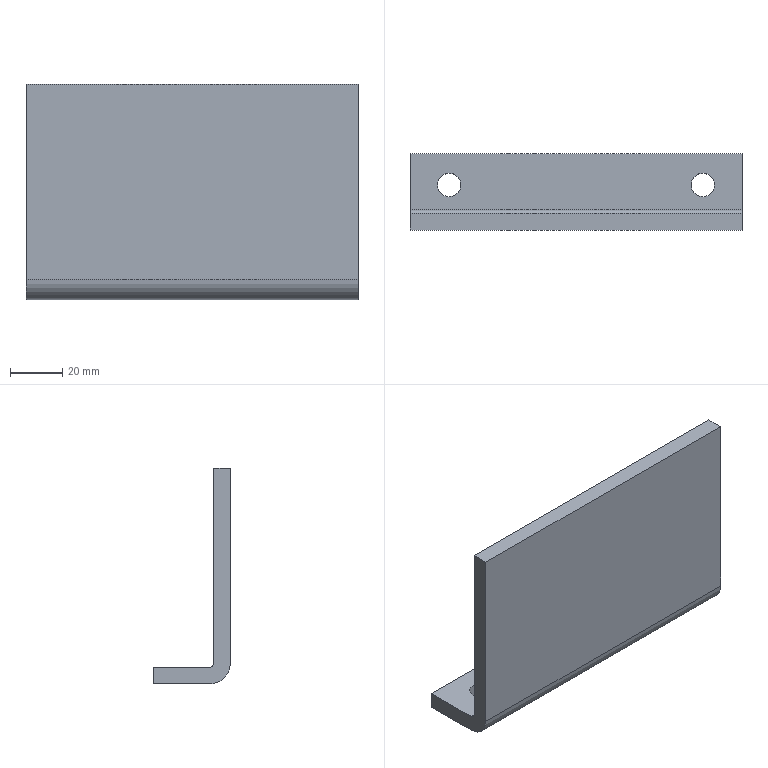Part | STEP file | 1_id706_x_t | 1 solid | 14 faces | box 127 x 29.369 x 82.55 mm | volume 82680 mm3 | plane 8 | cylinder 6 | commonest cylinder face diameters 9 x4 3.175 x1 15.875 x1
STEP:
#1=CARTESIAN_POINT('',(0.,0.,0.));
#2=DIRECTION('',(0.,0.,1.));
#3=DIRECTION('',(1.,0.,0.));
#4=AXIS2_PLACEMENT_3D('',#1,#2,#3);
#5=CARTESIAN_POINT('',(412.638,-208.869,-45.55));
#6=VERTEX_POINT('',#5);
#7=CARTESIAN_POINT('',(412.638,-202.519,-45.55));
#8=VERTEX_POINT('',#7);
#9=CARTESIAN_POINT('',(412.638,-208.869,-45.55));
#10=DIRECTION('',(0.,1.,0.));
#11=VECTOR('',#10,1.);
#12=LINE('',#9,#11);
#13=CARTESIAN_POINT('',(476.138,-148.544,-45.55));
#14=DIRECTION('',(0.,0.,1.));
#15=DIRECTION('',(1.,0.,0.));
#16=AXIS2_PLACEMENT_3D('',#13,#14,#15);
#17=PLANE('',#16);
#18=CARTESIAN_POINT('',(-63.5,-60.325));
#19=DIRECTION('',(0.,1.));
#20=VECTOR('',#19,1.);
#21=LINE('',#18,#20);
#22=(GEOMETRIC_REPRESENTATION_CONTEXT(2)PARAMETRIC_REPRESENTATION_CONTEXT()REPRESENTATION_CONTEXT('',''));
#23=DEFINITIONAL_REPRESENTATION('',(#21),#22);
#24=PCURVE('',#17,#23);
#25=CARTESIAN_POINT('',(412.638,-148.544,-86.825));
#26=DIRECTION('',(-1.,0.,0.));
#27=DIRECTION('',(0.,-1.,0.));
#28=AXIS2_PLACEMENT_3D('',#25,#26,#27);
#29=PLANE('',#28);
#30=CARTESIAN_POINT('',(60.325,41.275));
#31=DIRECTION('',(-1.,0.));
#32=VECTOR('',#31,1.);
#33=LINE('',#30,#32);
#34=(GEOMETRIC_REPRESENTATION_CONTEXT(2)PARAMETRIC_REPRESENTATION_CONTEXT()REPRESENTATION_CONTEXT('',''));
#35=DEFINITIONAL_REPRESENTATION('',(#33),#34);
#36=PCURVE('',#29,#35);
#37=SURFACE_CURVE('',#12,(#24,#36),.PCURVE_S1.);
#38=EDGE_CURVE('',#6,#8,#37,.T.);
#39=ORIENTED_EDGE('',*,*,#38,.F.);
#40=CARTESIAN_POINT('',(539.638,-208.869,-45.55));
#41=VERTEX_POINT('',#40);
#42=CARTESIAN_POINT('',(412.638,-208.869,-45.55));
#43=DIRECTION('',(1.,0.,0.));
#44=VECTOR('',#43,1.);
#45=LINE('',#42,#44);
#46=CARTESIAN_POINT('',(-63.5,-60.325));
#47=DIRECTION('',(1.,0.));
#48=VECTOR('',#47,1.);
#49=LINE('',#46,#48);
#50=(GEOMETRIC_REPRESENTATION_CONTEXT(2)PARAMETRIC_REPRESENTATION_CONTEXT()REPRESENTATION_CONTEXT('',''));
#51=DEFINITIONAL_REPRESENTATION('',(#49),#50);
#52=PCURVE('',#17,#51);
#53=CARTESIAN_POINT('',(476.138,-208.869,-86.825));
#54=DIRECTION('',(0.,-1.,0.));
#55=DIRECTION('',(0.,0.,1.));
#56=AXIS2_PLACEMENT_3D('',#53,#54,#55);
#57=PLANE('',#56);
#58=CARTESIAN_POINT('',(41.275,63.5));
#59=DIRECTION('',(0.,-1.));
#60=VECTOR('',#59,1.);
#61=LINE('',#58,#60);
#62=(GEOMETRIC_REPRESENTATION_CONTEXT(2)PARAMETRIC_REPRESENTATION_CONTEXT()REPRESENTATION_CONTEXT('',''));
#63=DEFINITIONAL_REPRESENTATION('',(#61),#62);
#64=PCURVE('',#57,#63);
#65=SURFACE_CURVE('',#45,(#52,#64),.PCURVE_S1.);
#66=EDGE_CURVE('',#6,#41,#65,.T.);
#67=ORIENTED_EDGE('',*,*,#66,.T.);
#68=CARTESIAN_POINT('',(539.638,-202.519,-45.55));
#69=VERTEX_POINT('',#68);
#70=CARTESIAN_POINT('',(539.638,-208.869,-45.55));
#71=DIRECTION('',(0.,1.,0.));
#72=VECTOR('',#71,1.);
#73=LINE('',#70,#72);
#74=CARTESIAN_POINT('',(63.5,-60.325));
#75=DIRECTION('',(0.,1.));
#76=VECTOR('',#75,1.);
#77=LINE('',#74,#76);
#78=(GEOMETRIC_REPRESENTATION_CONTEXT(2)PARAMETRIC_REPRESENTATION_CONTEXT()REPRESENTATION_CONTEXT('',''));
#79=DEFINITIONAL_REPRESENTATION('',(#77),#78);
#80=PCURVE('',#17,#79);
#81=CARTESIAN_POINT('',(539.638,-148.544,-86.825));
#82=DIRECTION('',(1.,0.,0.));
#83=DIRECTION('',(0.,0.,-1.));
#84=AXIS2_PLACEMENT_3D('',#81,#82,#83);
#85=PLANE('',#84);
#86=CARTESIAN_POINT('',(-41.275,-60.325));
#87=DIRECTION('',(0.,1.));
#88=VECTOR('',#87,1.);
#89=LINE('',#86,#88);
#90=(GEOMETRIC_REPRESENTATION_CONTEXT(2)PARAMETRIC_REPRESENTATION_CONTEXT()REPRESENTATION_CONTEXT('',''));
#91=DEFINITIONAL_REPRESENTATION('',(#89),#90);
#92=PCURVE('',#85,#91);
#93=SURFACE_CURVE('',#73,(#80,#92),.PCURVE_S1.);
#94=EDGE_CURVE('',#41,#69,#93,.T.);
#95=ORIENTED_EDGE('',*,*,#94,.T.);
#96=CARTESIAN_POINT('',(412.638,-202.519,-45.55));
#97=DIRECTION('',(1.,0.,0.));
#98=VECTOR('',#97,1.);
#99=LINE('',#96,#98);
#100=CARTESIAN_POINT('',(-63.5,-53.975));
#101=DIRECTION('',(1.,0.));
#102=VECTOR('',#101,1.);
#103=LINE('',#100,#102);
#104=(GEOMETRIC_REPRESENTATION_CONTEXT(2)PARAMETRIC_REPRESENTATION_CONTEXT()REPRESENTATION_CONTEXT('',''));
#105=DEFINITIONAL_REPRESENTATION('',(#103),#104);
#106=PCURVE('',#17,#105);
#107=CARTESIAN_POINT('',(476.138,-202.519,-86.825));
#108=DIRECTION('',(0.,-1.,0.));
#109=DIRECTION('',(0.,0.,1.));
#110=AXIS2_PLACEMENT_3D('',#107,#108,#109);
#111=PLANE('',#110);
#112=CARTESIAN_POINT('',(41.275,63.5));
#113=DIRECTION('',(0.,-1.));
#114=VECTOR('',#113,1.);
#115=LINE('',#112,#114);
#116=(GEOMETRIC_REPRESENTATION_CONTEXT(2)PARAMETRIC_REPRESENTATION_CONTEXT()REPRESENTATION_CONTEXT('',''));
#117=DEFINITIONAL_REPRESENTATION('',(#115),#116);
#118=PCURVE('',#111,#117);
#119=SURFACE_CURVE('',#99,(#106,#118),.PCURVE_S1.);
#120=EDGE_CURVE('',#8,#69,#119,.T.);
#121=ORIENTED_EDGE('',*,*,#120,.F.);
#122=EDGE_LOOP('',(#39,#67,#95,#121));
#123=FACE_BOUND('',#122,.T.);
#124=ADVANCED_FACE('',(#123),#17,.T.);
#125=ORIENTED_EDGE('',*,*,#120,.T.);
#126=CARTESIAN_POINT('',(539.638,-202.519,-120.163));
#127=VERTEX_POINT('',#126);
#128=CARTESIAN_POINT('',(539.638,-202.519,-45.55));
#129=DIRECTION('',(0.,0.,-1.));
#130=VECTOR('',#129,1.);
#131=LINE('',#128,#130);
#132=CARTESIAN_POINT('',(41.275,-63.5));
#133=DIRECTION('',(-1.,0.));
#134=VECTOR('',#133,1.);
#135=LINE('',#132,#134);
#136=(GEOMETRIC_REPRESENTATION_CONTEXT(2)PARAMETRIC_REPRESENTATION_CONTEXT()REPRESENTATION_CONTEXT('',''));
#137=DEFINITIONAL_REPRESENTATION('',(#135),#136);
#138=PCURVE('',#111,#137);
#139=CARTESIAN_POINT('',(-41.275,-53.975));
#140=DIRECTION('',(1.,0.));
#141=VECTOR('',#140,1.);
#142=LINE('',#139,#141);
#143=(GEOMETRIC_REPRESENTATION_CONTEXT(2)PARAMETRIC_REPRESENTATION_CONTEXT()REPRESENTATION_CONTEXT('',''));
#144=DEFINITIONAL_REPRESENTATION('',(#142),#143);
#145=PCURVE('',#85,#144);
#146=SURFACE_CURVE('',#131,(#138,#145),.PCURVE_S1.);
#147=EDGE_CURVE('',#69,#127,#146,.T.);
#148=ORIENTED_EDGE('',*,*,#147,.T.);
#149=CARTESIAN_POINT('',(412.638,-202.519,-120.163));
#150=VERTEX_POINT('',#149);
#151=CARTESIAN_POINT('',(412.638,-202.519,-120.163));
#152=DIRECTION('',(1.,0.,0.));
#153=VECTOR('',#152,1.);
#154=LINE('',#151,#153);
#155=CARTESIAN_POINT('',(-33.337,63.5));
#156=DIRECTION('',(0.,-1.));
#157=VECTOR('',#156,1.);
#158=LINE('',#155,#157);
#159=(GEOMETRIC_REPRESENTATION_CONTEXT(2)PARAMETRIC_REPRESENTATION_CONTEXT()REPRESENTATION_CONTEXT('',''));
#160=DEFINITIONAL_REPRESENTATION('',(#158),#159);
#161=PCURVE('',#111,#160);
#162=CARTESIAN_POINT('',(476.138,-200.931,-120.163));
#163=DIRECTION('',(1.,0.,0.));
#164=DIRECTION('',(0.,-1.,0.));
#165=AXIS2_PLACEMENT_3D('',#162,#163,#164);
#166=CYLINDRICAL_SURFACE('',#165,1.587);
#167=CARTESIAN_POINT('',(0.,-63.5));
#168=DIRECTION('',(0.,1.));
#169=VECTOR('',#168,1.);
#170=LINE('',#167,#169);
#171=(GEOMETRIC_REPRESENTATION_CONTEXT(2)PARAMETRIC_REPRESENTATION_CONTEXT()REPRESENTATION_CONTEXT('',''));
#172=DEFINITIONAL_REPRESENTATION('',(#170),#171);
#173=PCURVE('',#166,#172);
#174=SURFACE_CURVE('',#154,(#161,#173),.PCURVE_S1.);
#175=EDGE_CURVE('',#150,#127,#174,.T.);
#176=ORIENTED_EDGE('',*,*,#175,.F.);
#177=CARTESIAN_POINT('',(412.638,-202.519,-120.163));
#178=DIRECTION('',(0.,0.,1.));
#179=VECTOR('',#178,1.);
#180=LINE('',#177,#179);
#181=CARTESIAN_POINT('',(-33.337,63.5));
#182=DIRECTION('',(1.,0.));
#183=VECTOR('',#182,1.);
#184=LINE('',#181,#183);
#185=(GEOMETRIC_REPRESENTATION_CONTEXT(2)PARAMETRIC_REPRESENTATION_CONTEXT()REPRESENTATION_CONTEXT('',''));
#186=DEFINITIONAL_REPRESENTATION('',(#184),#185);
#187=PCURVE('',#111,#186);
#188=CARTESIAN_POINT('',(53.975,-33.337));
#189=DIRECTION('',(0.,1.));
#190=VECTOR('',#189,1.);
#191=LINE('',#188,#190);
#192=(GEOMETRIC_REPRESENTATION_CONTEXT(2)PARAMETRIC_REPRESENTATION_CONTEXT()REPRESENTATION_CONTEXT('',''));
#193=DEFINITIONAL_REPRESENTATION('',(#191),#192);
#194=PCURVE('',#29,#193);
#195=SURFACE_CURVE('',#180,(#187,#194),.PCURVE_S1.);
#196=EDGE_CURVE('',#150,#8,#195,.T.);
#197=ORIENTED_EDGE('',*,*,#196,.T.);
#198=EDGE_LOOP('',(#125,#148,#176,#197));
#199=FACE_BOUND('',#198,.T.);
#200=ADVANCED_FACE('',(#199),#111,.F.);
#201=CARTESIAN_POINT('',(412.638,-200.931,-128.1));
#202=VERTEX_POINT('',#201);
#203=CARTESIAN_POINT('',(412.638,-179.5,-128.1));
#204=VERTEX_POINT('',#203);
#205=CARTESIAN_POINT('',(412.638,-200.931,-128.1));
#206=DIRECTION('',(0.,1.,0.));
#207=VECTOR('',#206,1.);
#208=LINE('',#205,#207);
#209=CARTESIAN_POINT('',(52.388,-41.275));
#210=DIRECTION('',(-1.,0.));
#211=VECTOR('',#210,1.);
#212=LINE('',#209,#211);
#213=(GEOMETRIC_REPRESENTATION_CONTEXT(2)PARAMETRIC_REPRESENTATION_CONTEXT()REPRESENTATION_CONTEXT('',''));
#214=DEFINITIONAL_REPRESENTATION('',(#212),#213);
#215=PCURVE('',#29,#214);
#216=CARTESIAN_POINT('',(476.138,-148.544,-128.1));
#217=DIRECTION('',(0.,0.,-1.));
#218=DIRECTION('',(0.,1.,0.));
#219=AXIS2_PLACEMENT_3D('',#216,#217,#218);
#220=PLANE('',#219);
#221=CARTESIAN_POINT('',(-52.388,-63.5));
#222=DIRECTION('',(1.,0.));
#223=VECTOR('',#222,1.);
#224=LINE('',#221,#223);
#225=(GEOMETRIC_REPRESENTATION_CONTEXT(2)PARAMETRIC_REPRESENTATION_CONTEXT()REPRESENTATION_CONTEXT('',''));
#226=DEFINITIONAL_REPRESENTATION('',(#224),#225);
#227=PCURVE('',#220,#226);
#228=SURFACE_CURVE('',#208,(#215,#227),.PCURVE_S1.);
#229=EDGE_CURVE('',#202,#204,#228,.T.);
#230=ORIENTED_EDGE('',*,*,#229,.F.);
#231=CARTESIAN_POINT('',(412.638,-208.869,-120.163));
#232=VERTEX_POINT('',#231);
#233=CARTESIAN_POINT('',(412.638,-200.931,-120.163));
#234=DIRECTION('',(-1.,0.,0.));
#235=DIRECTION('',(0.,0.,-1.));
#236=AXIS2_PLACEMENT_3D('',#233,#234,#235);
#237=CIRCLE('',#236,7.938);
#238=CARTESIAN_POINT('',(52.388,-33.337));
#239=DIRECTION('',(0.,-1.));
#240=AXIS2_PLACEMENT_2D('',#238,#239);
#241=CIRCLE('',#240,7.938);
#242=(GEOMETRIC_REPRESENTATION_CONTEXT(2)PARAMETRIC_REPRESENTATION_CONTEXT()REPRESENTATION_CONTEXT('',''));
#243=DEFINITIONAL_REPRESENTATION('',(#241),#242);
#244=PCURVE('',#29,#243);
#245=CARTESIAN_POINT('',(476.138,-200.931,-120.163));
#246=DIRECTION('',(-1.,0.,0.));
#247=DIRECTION('',(0.,1.,0.));
#248=AXIS2_PLACEMENT_3D('',#245,#246,#247);
#249=CYLINDRICAL_SURFACE('',#248,7.938);
#250=CARTESIAN_POINT('',(1.571,63.5));
#251=DIRECTION('',(1.,0.));
#252=VECTOR('',#251,1.);
#253=LINE('',#250,#252);
#254=(GEOMETRIC_REPRESENTATION_CONTEXT(2)PARAMETRIC_REPRESENTATION_CONTEXT()REPRESENTATION_CONTEXT('',''));
#255=DEFINITIONAL_REPRESENTATION('',(#253),#254);
#256=PCURVE('',#249,#255);
#257=SURFACE_CURVE('',#237,(#244,#256),.PCURVE_S1.);
#258=EDGE_CURVE('',#202,#232,#257,.T.);
#259=ORIENTED_EDGE('',*,*,#258,.T.);
#260=CARTESIAN_POINT('',(412.638,-208.869,-120.163));
#261=DIRECTION('',(0.,0.,1.));
#262=VECTOR('',#261,1.);
#263=LINE('',#260,#262);
#264=CARTESIAN_POINT('',(60.325,-33.337));
#265=DIRECTION('',(0.,1.));
#266=VECTOR('',#265,1.);
#267=LINE('',#264,#266);
#268=(GEOMETRIC_REPRESENTATION_CONTEXT(2)PARAMETRIC_REPRESENTATION_CONTEXT()REPRESENTATION_CONTEXT('',''));
#269=DEFINITIONAL_REPRESENTATION('',(#267),#268);
#270=PCURVE('',#29,#269);
#271=CARTESIAN_POINT('',(-33.337,63.5));
#272=DIRECTION('',(1.,0.));
#273=VECTOR('',#272,1.);
#274=LINE('',#271,#273);
#275=(GEOMETRIC_REPRESENTATION_CONTEXT(2)PARAMETRIC_REPRESENTATION_CONTEXT()REPRESENTATION_CONTEXT('',''));
#276=DEFINITIONAL_REPRESENTATION('',(#274),#275);
#277=PCURVE('',#57,#276);
#278=SURFACE_CURVE('',#263,(#270,#277),.PCURVE_S1.);
#279=EDGE_CURVE('',#232,#6,#278,.T.);
#280=ORIENTED_EDGE('',*,*,#279,.T.);
#281=ORIENTED_EDGE('',*,*,#38,.T.);
#282=ORIENTED_EDGE('',*,*,#196,.F.);
#283=CARTESIAN_POINT('',(412.638,-200.931,-121.75));
#284=VERTEX_POINT('',#283);
#285=CARTESIAN_POINT('',(412.638,-200.931,-120.163));
#286=DIRECTION('',(1.,0.,0.));
#287=DIRECTION('',(0.,-1.,0.));
#288=AXIS2_PLACEMENT_3D('',#285,#286,#287);
#289=CIRCLE('',#288,1.587);
#290=CARTESIAN_POINT('',(53.975,-33.337));
#291=CARTESIAN_POINT('',(53.975,-36.087));
#292=CARTESIAN_POINT('',(51.594,-34.712));
#293=CARTESIAN_POINT('',(49.212,-33.337));
#294=CARTESIAN_POINT('',(51.594,-31.963));
#295=CARTESIAN_POINT('',(53.975,-30.588));
#296=CARTESIAN_POINT('',(53.975,-33.337));
#297=(BOUNDED_CURVE()B_SPLINE_CURVE(2,(#290,#291,#292,#293,#294,#295,#296),.UNSPECIFIED.,.T.,.F.)B_SPLINE_CURVE_WITH_KNOTS((1,2,2,2,2,1),(-2.094,0.,2.094,4.189,6.283,8.378),.UNSPECIFIED.)CURVE()GEOMETRIC_REPRESENTATION_ITEM()RATIONAL_B_SPLINE_CURVE((1.,0.5,1.,0.5,1.,0.5,1.))REPRESENTATION_ITEM(''));
#298=(GEOMETRIC_REPRESENTATION_CONTEXT(2)PARAMETRIC_REPRESENTATION_CONTEXT()REPRESENTATION_CONTEXT('',''));
#299=DEFINITIONAL_REPRESENTATION('',(#297),#298);
#300=PCURVE('',#29,#299);
#301=CARTESIAN_POINT('',(0.,-63.5));
#302=DIRECTION('',(1.,0.));
#303=VECTOR('',#302,1.);
#304=LINE('',#301,#303);
#305=(GEOMETRIC_REPRESENTATION_CONTEXT(2)PARAMETRIC_REPRESENTATION_CONTEXT()REPRESENTATION_CONTEXT('',''));
#306=DEFINITIONAL_REPRESENTATION('',(#304),#305);
#307=PCURVE('',#166,#306);
#308=SURFACE_CURVE('',#289,(#300,#307),.PCURVE_S1.);
#309=EDGE_CURVE('',#150,#284,#308,.T.);
#310=ORIENTED_EDGE('',*,*,#309,.T.);
#311=CARTESIAN_POINT('',(412.638,-179.5,-121.75));
#312=VERTEX_POINT('',#311);
#313=CARTESIAN_POINT('',(412.638,-200.931,-121.75));
#314=DIRECTION('',(0.,1.,0.));
#315=VECTOR('',#314,1.);
#316=LINE('',#313,#315);
#317=CARTESIAN_POINT('',(52.388,-34.925));
#318=DIRECTION('',(-1.,0.));
#319=VECTOR('',#318,1.);
#320=LINE('',#317,#319);
#321=(GEOMETRIC_REPRESENTATION_CONTEXT(2)PARAMETRIC_REPRESENTATION_CONTEXT()REPRESENTATION_CONTEXT('',''));
#322=DEFINITIONAL_REPRESENTATION('',(#320),#321);
#323=PCURVE('',#29,#322);
#324=CARTESIAN_POINT('',(476.138,-148.544,-121.75));
#325=DIRECTION('',(0.,0.,-1.));
#326=DIRECTION('',(0.,1.,0.));
#327=AXIS2_PLACEMENT_3D('',#324,#325,#326);
#328=PLANE('',#327);
#329=CARTESIAN_POINT('',(-52.388,-63.5));
#330=DIRECTION('',(1.,0.));
#331=VECTOR('',#330,1.);
#332=LINE('',#329,#331);
#333=(GEOMETRIC_REPRESENTATION_CONTEXT(2)PARAMETRIC_REPRESENTATION_CONTEXT()REPRESENTATION_CONTEXT('',''));
#334=DEFINITIONAL_REPRESENTATION('',(#332),#333);
#335=PCURVE('',#328,#334);
#336=SURFACE_CURVE('',#316,(#323,#335),.PCURVE_S1.);
#337=EDGE_CURVE('',#284,#312,#336,.T.);
#338=ORIENTED_EDGE('',*,*,#337,.T.);
#339=CARTESIAN_POINT('',(412.638,-179.5,-128.1));
#340=DIRECTION('',(0.,0.,1.));
#341=VECTOR('',#340,1.);
#342=LINE('',#339,#341);
#343=CARTESIAN_POINT('',(30.956,-41.275));
#344=DIRECTION('',(0.,1.));
#345=VECTOR('',#344,1.);
#346=LINE('',#343,#345);
#347=(GEOMETRIC_REPRESENTATION_CONTEXT(2)PARAMETRIC_REPRESENTATION_CONTEXT()REPRESENTATION_CONTEXT('',''));
#348=DEFINITIONAL_REPRESENTATION('',(#346),#347);
#349=PCURVE('',#29,#348);
#350=CARTESIAN_POINT('',(368.95,-179.5,-128.1));
#351=DIRECTION('',(0.,-1.,0.));
#352=DIRECTION('',(0.,0.,1.));
#353=AXIS2_PLACEMENT_3D('',#350,#351,#352);
#354=PLANE('',#353);
#355=CARTESIAN_POINT('',(0.,-43.688));
#356=DIRECTION('',(1.,0.));
#357=VECTOR('',#356,1.);
#358=LINE('',#355,#357);
#359=(GEOMETRIC_REPRESENTATION_CONTEXT(2)PARAMETRIC_REPRESENTATION_CONTEXT()REPRESENTATION_CONTEXT('',''));
#360=DEFINITIONAL_REPRESENTATION('',(#358),#359);
#361=PCURVE('',#354,#360);
#362=SURFACE_CURVE('',#342,(#349,#361),.PCURVE_S1.);
#363=EDGE_CURVE('',#204,#312,#362,.T.);
#364=ORIENTED_EDGE('',*,*,#363,.F.);
#365=EDGE_LOOP('',(#230,#259,#280,#281,#282,#310,#338,#364));
#366=FACE_BOUND('',#365,.T.);
#367=ADVANCED_FACE('',(#366),#29,.T.);
#368=CARTESIAN_POINT('',(539.638,-179.5,-121.75));
#369=VERTEX_POINT('',#368);
#370=CARTESIAN_POINT('',(539.638,-179.5,-121.75));
#371=DIRECTION('',(-1.,0.,0.));
#372=VECTOR('',#371,1.);
#373=LINE('',#370,#372);
#374=CARTESIAN_POINT('',(6.35,-170.688));
#375=DIRECTION('',(0.,1.));
#376=VECTOR('',#375,1.);
#377=LINE('',#374,#376);
#378=(GEOMETRIC_REPRESENTATION_CONTEXT(2)PARAMETRIC_REPRESENTATION_CONTEXT()REPRESENTATION_CONTEXT('',''));
#379=DEFINITIONAL_REPRESENTATION('',(#377),#378);
#380=PCURVE('',#354,#379);
#381=CARTESIAN_POINT('',(-30.956,63.5));
#382=DIRECTION('',(0.,-1.));
#383=VECTOR('',#382,1.);
#384=LINE('',#381,#383);
#385=(GEOMETRIC_REPRESENTATION_CONTEXT(2)PARAMETRIC_REPRESENTATION_CONTEXT()REPRESENTATION_CONTEXT('',''));
#386=DEFINITIONAL_REPRESENTATION('',(#384),#385);
#387=PCURVE('',#328,#386);
#388=SURFACE_CURVE('',#373,(#380,#387),.PCURVE_S1.);
#389=EDGE_CURVE('',#369,#312,#388,.T.);
#390=ORIENTED_EDGE('',*,*,#389,.F.);
#391=CARTESIAN_POINT('',(539.638,-179.5,-128.1));
#392=VERTEX_POINT('',#391);
#393=CARTESIAN_POINT('',(539.638,-179.5,-121.75));
#394=DIRECTION('',(0.,0.,-1.));
#395=VECTOR('',#394,1.);
#396=LINE('',#393,#395);
#397=CARTESIAN_POINT('',(6.35,-170.688));
#398=DIRECTION('',(-1.,0.));
#399=VECTOR('',#398,1.);
#400=LINE('',#397,#399);
#401=(GEOMETRIC_REPRESENTATION_CONTEXT(2)PARAMETRIC_REPRESENTATION_CONTEXT()REPRESENTATION_CONTEXT('',''));
#402=DEFINITIONAL_REPRESENTATION('',(#400),#401);
#403=PCURVE('',#354,#402);
#404=CARTESIAN_POINT('',(34.925,-30.956));
#405=DIRECTION('',(1.,0.));
#406=VECTOR('',#405,1.);
#407=LINE('',#404,#406);
#408=(GEOMETRIC_REPRESENTATION_CONTEXT(2)PARAMETRIC_REPRESENTATION_CONTEXT()REPRESENTATION_CONTEXT('',''));
#409=DEFINITIONAL_REPRESENTATION('',(#407),#408);
#410=PCURVE('',#85,#409);
#411=SURFACE_CURVE('',#396,(#403,#410),.PCURVE_S1.);
#412=EDGE_CURVE('',#369,#392,#411,.T.);
#413=ORIENTED_EDGE('',*,*,#412,.T.);
#414=CARTESIAN_POINT('',(539.638,-179.5,-128.1));
#415=DIRECTION('',(-1.,0.,0.));
#416=VECTOR('',#415,1.);
#417=LINE('',#414,#416);
#418=CARTESIAN_POINT('',(0.,-170.688));
#419=DIRECTION('',(0.,1.));
#420=VECTOR('',#419,1.);
#421=LINE('',#418,#420);
#422=(GEOMETRIC_REPRESENTATION_CONTEXT(2)PARAMETRIC_REPRESENTATION_CONTEXT()REPRESENTATION_CONTEXT('',''));
#423=DEFINITIONAL_REPRESENTATION('',(#421),#422);
#424=PCURVE('',#354,#423);
#425=CARTESIAN_POINT('',(-30.956,63.5));
#426=DIRECTION('',(0.,-1.));
#427=VECTOR('',#426,1.);
#428=LINE('',#425,#427);
#429=(GEOMETRIC_REPRESENTATION_CONTEXT(2)PARAMETRIC_REPRESENTATION_CONTEXT()REPRESENTATION_CONTEXT('',''));
#430=DEFINITIONAL_REPRESENTATION('',(#428),#429);
#431=PCURVE('',#220,#430);
#432=SURFACE_CURVE('',#417,(#424,#431),.PCURVE_S1.);
#433=EDGE_CURVE('',#392,#204,#432,.T.);
#434=ORIENTED_EDGE('',*,*,#433,.T.);
#435=ORIENTED_EDGE('',*,*,#363,.T.);
#436=EDGE_LOOP('',(#390,#413,#434,#435));
#437=FACE_BOUND('',#436,.T.);
#438=ADVANCED_FACE('',(#437),#354,.F.);
#439=CARTESIAN_POINT('',(539.638,-200.931,-128.1));
#440=VERTEX_POINT('',#439);
#441=CARTESIAN_POINT('',(539.638,-200.931,-128.1));
#442=DIRECTION('',(0.,1.,0.));
#443=VECTOR('',#442,1.);
#444=LINE('',#441,#443);
#445=CARTESIAN_POINT('',(-52.388,63.5));
#446=DIRECTION('',(1.,0.));
#447=VECTOR('',#446,1.);
#448=LINE('',#445,#447);
#449=(GEOMETRIC_REPRESENTATION_CONTEXT(2)PARAMETRIC_REPRESENTATION_CONTEXT()REPRESENTATION_CONTEXT('',''));
#450=DEFINITIONAL_REPRESENTATION('',(#448),#449);
#451=PCURVE('',#220,#450);
#452=CARTESIAN_POINT('',(41.275,-52.388));
#453=DIRECTION('',(0.,1.));
#454=VECTOR('',#453,1.);
#455=LINE('',#452,#454);
#456=(GEOMETRIC_REPRESENTATION_CONTEXT(2)PARAMETRIC_REPRESENTATION_CONTEXT()REPRESENTATION_CONTEXT('',''));
#457=DEFINITIONAL_REPRESENTATION('',(#455),#456);
#458=PCURVE('',#85,#457);
#459=SURFACE_CURVE('',#444,(#451,#458),.PCURVE_S1.);
#460=EDGE_CURVE('',#440,#392,#459,.T.);
#461=ORIENTED_EDGE('',*,*,#460,.F.);
#462=CARTESIAN_POINT('',(412.638,-200.931,-128.1));
#463=DIRECTION('',(1.,0.,0.));
#464=VECTOR('',#463,1.);
#465=LINE('',#462,#464);
#466=CARTESIAN_POINT('',(-52.388,-63.5));
#467=DIRECTION('',(0.,1.));
#468=VECTOR('',#467,1.);
#469=LINE('',#466,#468);
#470=(GEOMETRIC_REPRESENTATION_CONTEXT(2)PARAMETRIC_REPRESENTATION_CONTEXT()REPRESENTATION_CONTEXT('',''));
#471=DEFINITIONAL_REPRESENTATION('',(#469),#470);
#472=PCURVE('',#220,#471);
#473=CARTESIAN_POINT('',(1.571,63.5));
#474=DIRECTION('',(0.,-1.));
#475=VECTOR('',#474,1.);
#476=LINE('',#473,#475);
#477=(GEOMETRIC_REPRESENTATION_CONTEXT(2)PARAMETRIC_REPRESENTATION_CONTEXT()REPRESENTATION_CONTEXT('',''));
#478=DEFINITIONAL_REPRESENTATION('',(#476),#477);
#479=PCURVE('',#249,#478);
#480=SURFACE_CURVE('',#465,(#472,#479),.PCURVE_S1.);
#481=EDGE_CURVE('',#202,#440,#480,.T.);
#482=ORIENTED_EDGE('',*,*,#481,.F.);
#483=ORIENTED_EDGE('',*,*,#229,.T.);
#484=ORIENTED_EDGE('',*,*,#433,.F.);
#485=EDGE_LOOP('',(#461,#482,#483,#484));
#486=FACE_BOUND('',#485,.T.);
#487=CARTESIAN_POINT('',(432.138,-191.5,-128.1));
#488=VERTEX_POINT('',#487);
#489=CARTESIAN_POINT('',(423.138,-191.5,-128.1));
#490=VERTEX_POINT('',#489);
#491=CARTESIAN_POINT('',(427.638,-191.5,-128.1));
#492=DIRECTION('',(0.,0.,1.));
#493=DIRECTION('',(1.,0.,0.));
#494=AXIS2_PLACEMENT_3D('',#491,#492,#493);
#495=CIRCLE('',#494,4.5);
#496=CARTESIAN_POINT('',(-42.956,-44.));
#497=CARTESIAN_POINT('',(-35.162,-44.));
#498=CARTESIAN_POINT('',(-39.059,-50.75));
#499=CARTESIAN_POINT('',(-42.956,-57.5));
#500=CARTESIAN_POINT('',(-46.853,-50.75));
#501=CARTESIAN_POINT('',(-50.75,-44.));
#502=CARTESIAN_POINT('',(-42.956,-44.));
#503=(BOUNDED_CURVE()B_SPLINE_CURVE(2,(#496,#497,#498,#499,#500,#501,#502),.UNSPECIFIED.,.T.,.F.)B_SPLINE_CURVE_WITH_KNOTS((1,2,2,2,2,1),(-2.094,0.,2.094,4.189,6.283,8.378),.UNSPECIFIED.)CURVE()GEOMETRIC_REPRESENTATION_ITEM()RATIONAL_B_SPLINE_CURVE((1.,0.5,1.,0.5,1.,0.5,1.))REPRESENTATION_ITEM(''));
#504=(GEOMETRIC_REPRESENTATION_CONTEXT(2)PARAMETRIC_REPRESENTATION_CONTEXT()REPRESENTATION_CONTEXT('',''));
#505=DEFINITIONAL_REPRESENTATION('',(#503),#504);
#506=PCURVE('',#220,#505);
#507=CARTESIAN_POINT('',(427.638,-191.5,-112.75));
#508=DIRECTION('',(0.,0.,-1.));
#509=DIRECTION('',(1.,0.,0.));
#510=AXIS2_PLACEMENT_3D('',#507,#508,#509);
#511=CYLINDRICAL_SURFACE('',#510,4.5);
#512=CARTESIAN_POINT('',(6.283,15.35));
#513=DIRECTION('',(-1.,0.));
#514=VECTOR('',#513,1.);
#515=LINE('',#512,#514);
#516=(GEOMETRIC_REPRESENTATION_CONTEXT(2)PARAMETRIC_REPRESENTATION_CONTEXT()REPRESENTATION_CONTEXT('',''));
#517=DEFINITIONAL_REPRESENTATION('',(#515),#516);
#518=PCURVE('',#511,#517);
#519=SURFACE_CURVE('',#495,(#506,#518),.PCURVE_S1.);
#520=EDGE_CURVE('',#488,#490,#519,.T.);
#521=ORIENTED_EDGE('',*,*,#520,.T.);
#522=CARTESIAN_POINT('',(427.638,-191.5,-128.1));
#523=DIRECTION('',(0.,0.,1.));
#524=DIRECTION('',(-1.,0.,0.));
#525=AXIS2_PLACEMENT_3D('',#522,#523,#524);
#526=CIRCLE('',#525,4.5);
#527=CARTESIAN_POINT('',(-42.956,-53.));
#528=CARTESIAN_POINT('',(-50.75,-53.));
#529=CARTESIAN_POINT('',(-46.853,-46.25));
#530=CARTESIAN_POINT('',(-42.956,-39.5));
#531=CARTESIAN_POINT('',(-39.059,-46.25));
#532=CARTESIAN_POINT('',(-35.162,-53.));
#533=CARTESIAN_POINT('',(-42.956,-53.));
#534=(BOUNDED_CURVE()B_SPLINE_CURVE(2,(#527,#528,#529,#530,#531,#532,#533),.UNSPECIFIED.,.T.,.F.)B_SPLINE_CURVE_WITH_KNOTS((1,2,2,2,2,1),(-2.094,0.,2.094,4.189,6.283,8.378),.UNSPECIFIED.)CURVE()GEOMETRIC_REPRESENTATION_ITEM()RATIONAL_B_SPLINE_CURVE((1.,0.5,1.,0.5,1.,0.5,1.))REPRESENTATION_ITEM(''));
#535=(GEOMETRIC_REPRESENTATION_CONTEXT(2)PARAMETRIC_REPRESENTATION_CONTEXT()REPRESENTATION_CONTEXT('',''));
#536=DEFINITIONAL_REPRESENTATION('',(#534),#535);
#537=PCURVE('',#220,#536);
#538=CARTESIAN_POINT('',(427.638,-191.5,-112.75));
#539=DIRECTION('',(0.,0.,-1.));
#540=DIRECTION('',(1.,0.,0.));
#541=AXIS2_PLACEMENT_3D('',#538,#539,#540);
#542=CYLINDRICAL_SURFACE('',#541,4.5);
#543=CARTESIAN_POINT('',(3.142,15.35));
#544=DIRECTION('',(-1.,0.));
#545=VECTOR('',#544,1.);
#546=LINE('',#543,#545);
#547=(GEOMETRIC_REPRESENTATION_CONTEXT(2)PARAMETRIC_REPRESENTATION_CONTEXT()REPRESENTATION_CONTEXT('',''));
#548=DEFINITIONAL_REPRESENTATION('',(#546),#547);
#549=PCURVE('',#542,#548);
#550=SURFACE_CURVE('',#526,(#537,#549),.PCURVE_S1.);
#551=EDGE_CURVE('',#490,#488,#550,.T.);
#552=ORIENTED_EDGE('',*,*,#551,.T.);
#553=EDGE_LOOP('',(#521,#552));
#554=FACE_BOUND('',#553,.T.);
#555=CARTESIAN_POINT('',(529.138,-191.5,-128.1));
#556=VERTEX_POINT('',#555);
#557=CARTESIAN_POINT('',(520.138,-191.5,-128.1));
#558=VERTEX_POINT('',#557);
#559=CARTESIAN_POINT('',(524.638,-191.5,-128.1));
#560=DIRECTION('',(0.,0.,1.));
#561=DIRECTION('',(1.,0.,0.));
#562=AXIS2_PLACEMENT_3D('',#559,#560,#561);
#563=CIRCLE('',#562,4.5);
#564=CARTESIAN_POINT('',(-42.956,53.));
#565=CARTESIAN_POINT('',(-35.162,53.));
#566=CARTESIAN_POINT('',(-39.059,46.25));
#567=CARTESIAN_POINT('',(-42.956,39.5));
#568=CARTESIAN_POINT('',(-46.853,46.25));
#569=CARTESIAN_POINT('',(-50.75,53.));
#570=CARTESIAN_POINT('',(-42.956,53.));
#571=(BOUNDED_CURVE()B_SPLINE_CURVE(2,(#564,#565,#566,#567,#568,#569,#570),.UNSPECIFIED.,.T.,.F.)B_SPLINE_CURVE_WITH_KNOTS((1,2,2,2,2,1),(-2.094,0.,2.094,4.189,6.283,8.378),.UNSPECIFIED.)CURVE()GEOMETRIC_REPRESENTATION_ITEM()RATIONAL_B_SPLINE_CURVE((1.,0.5,1.,0.5,1.,0.5,1.))REPRESENTATION_ITEM(''));
#572=(GEOMETRIC_REPRESENTATION_CONTEXT(2)PARAMETRIC_REPRESENTATION_CONTEXT()REPRESENTATION_CONTEXT('',''));
#573=DEFINITIONAL_REPRESENTATION('',(#571),#572);
#574=PCURVE('',#220,#573);
#575=CARTESIAN_POINT('',(524.638,-191.5,-112.75));
#576=DIRECTION('',(0.,0.,-1.));
#577=DIRECTION('',(-1.,0.,0.));
#578=AXIS2_PLACEMENT_3D('',#575,#576,#577);
#579=CYLINDRICAL_SURFACE('',#578,4.5);
#580=CARTESIAN_POINT('',(3.142,15.35));
#581=DIRECTION('',(-1.,0.));
#582=VECTOR('',#581,1.);
#583=LINE('',#580,#582);
#584=(GEOMETRIC_REPRESENTATION_CONTEXT(2)PARAMETRIC_REPRESENTATION_CONTEXT()REPRESENTATION_CONTEXT('',''));
#585=DEFINITIONAL_REPRESENTATION('',(#583),#584);
#586=PCURVE('',#579,#585);
#587=SURFACE_CURVE('',#563,(#574,#586),.PCURVE_S1.);
#588=EDGE_CURVE('',#556,#558,#587,.T.);
#589=ORIENTED_EDGE('',*,*,#588,.T.);
#590=CARTESIAN_POINT('',(524.638,-191.5,-128.1));
#591=DIRECTION('',(0.,0.,1.));
#592=DIRECTION('',(-1.,0.,0.));
#593=AXIS2_PLACEMENT_3D('',#590,#591,#592);
#594=CIRCLE('',#593,4.5);
#595=CARTESIAN_POINT('',(-42.956,44.));
#596=CARTESIAN_POINT('',(-50.75,44.));
#597=CARTESIAN_POINT('',(-46.853,50.75));
#598=CARTESIAN_POINT('',(-42.956,57.5));
#599=CARTESIAN_POINT('',(-39.059,50.75));
#600=CARTESIAN_POINT('',(-35.162,44.));
#601=CARTESIAN_POINT('',(-42.956,44.));
#602=(BOUNDED_CURVE()B_SPLINE_CURVE(2,(#595,#596,#597,#598,#599,#600,#601),.UNSPECIFIED.,.T.,.F.)B_SPLINE_CURVE_WITH_KNOTS((1,2,2,2,2,1),(-2.094,0.,2.094,4.189,6.283,8.378),.UNSPECIFIED.)CURVE()GEOMETRIC_REPRESENTATION_ITEM()RATIONAL_B_SPLINE_CURVE((1.,0.5,1.,0.5,1.,0.5,1.))REPRESENTATION_ITEM(''));
#603=(GEOMETRIC_REPRESENTATION_CONTEXT(2)PARAMETRIC_REPRESENTATION_CONTEXT()REPRESENTATION_CONTEXT('',''));
#604=DEFINITIONAL_REPRESENTATION('',(#602),#603);
#605=PCURVE('',#220,#604);
#606=CARTESIAN_POINT('',(524.638,-191.5,-112.75));
#607=DIRECTION('',(0.,0.,-1.));
#608=DIRECTION('',(-1.,0.,0.));
#609=AXIS2_PLACEMENT_3D('',#606,#607,#608);
#610=CYLINDRICAL_SURFACE('',#609,4.5);
#611=CARTESIAN_POINT('',(6.283,15.35));
#612=DIRECTION('',(-1.,0.));
#613=VECTOR('',#612,1.);
#614=LINE('',#611,#613);
#615=(GEOMETRIC_REPRESENTATION_CONTEXT(2)PARAMETRIC_REPRESENTATION_CONTEXT()REPRESENTATION_CONTEXT('',''));
#616=DEFINITIONAL_REPRESENTATION('',(#614),#615);
#617=PCURVE('',#610,#616);
#618=SURFACE_CURVE('',#594,(#605,#617),.PCURVE_S1.);
#619=EDGE_CURVE('',#558,#556,#618,.T.);
#620=ORIENTED_EDGE('',*,*,#619,.T.);
#621=EDGE_LOOP('',(#589,#620));
#622=FACE_BOUND('',#621,.T.);
#623=ADVANCED_FACE('',(#486,#554,#622),#220,.T.);
#624=ORIENTED_EDGE('',*,*,#551,.T.);
#625=CARTESIAN_POINT('',(432.138,-191.5,-121.75));
#626=VERTEX_POINT('',#625);
#627=CARTESIAN_POINT('',(432.138,-191.5,-121.75));
#628=DIRECTION('',(0.,0.,-1.));
#629=VECTOR('',#628,1.);
#630=LINE('',#627,#629);
#631=CARTESIAN_POINT('',(0.,9.));
#632=DIRECTION('',(0.,1.));
#633=VECTOR('',#632,1.);
#634=LINE('',#631,#633);
#635=(GEOMETRIC_REPRESENTATION_CONTEXT(2)PARAMETRIC_REPRESENTATION_CONTEXT()REPRESENTATION_CONTEXT('',''));
#636=DEFINITIONAL_REPRESENTATION('',(#634),#635);
#637=PCURVE('',#542,#636);
#638=CARTESIAN_POINT('',(6.283,9.));
#639=DIRECTION('',(0.,1.));
#640=VECTOR('',#639,1.);
#641=LINE('',#638,#640);
#642=(GEOMETRIC_REPRESENTATION_CONTEXT(2)PARAMETRIC_REPRESENTATION_CONTEXT()REPRESENTATION_CONTEXT('',''));
#643=DEFINITIONAL_REPRESENTATION('',(#641),#642);
#644=PCURVE('',#511,#643);
#645=SURFACE_CURVE('',#630,(#637,#644),.PCURVE_S1.);
#646=EDGE_CURVE('',#626,#488,#645,.T.);
#647=ORIENTED_EDGE('',*,*,#646,.F.);
#648=CARTESIAN_POINT('',(423.138,-191.5,-121.75));
#649=VERTEX_POINT('',#648);
#650=CARTESIAN_POINT('',(427.638,-191.5,-121.75));
#651=DIRECTION('',(0.,0.,-1.));
#652=DIRECTION('',(1.,0.,0.));
#653=AXIS2_PLACEMENT_3D('',#650,#651,#652);
#654=CIRCLE('',#653,4.5);
#655=CARTESIAN_POINT('',(0.,9.));
#656=DIRECTION('',(1.,0.));
#657=VECTOR('',#656,1.);
#658=LINE('',#655,#657);
#659=(GEOMETRIC_REPRESENTATION_CONTEXT(2)PARAMETRIC_REPRESENTATION_CONTEXT()REPRESENTATION_CONTEXT('',''));
#660=DEFINITIONAL_REPRESENTATION('',(#658),#659);
#661=PCURVE('',#542,#660);
#662=CARTESIAN_POINT('',(-42.956,-48.5));
#663=DIRECTION('',(0.,1.));
#664=AXIS2_PLACEMENT_2D('',#662,#663);
#665=CIRCLE('',#664,4.5);
#666=(GEOMETRIC_REPRESENTATION_CONTEXT(2)PARAMETRIC_REPRESENTATION_CONTEXT()REPRESENTATION_CONTEXT('',''));
#667=DEFINITIONAL_REPRESENTATION('',(#665),#666);
#668=PCURVE('',#328,#667);
#669=SURFACE_CURVE('',#654,(#661,#668),.PCURVE_S1.);
#670=EDGE_CURVE('',#626,#649,#669,.T.);
#671=ORIENTED_EDGE('',*,*,#670,.T.);
#672=CARTESIAN_POINT('',(423.138,-191.5,-121.75));
#673=DIRECTION('',(0.,0.,1.));
#674=VECTOR('',#673,1.);
#675=LINE('',#672,#674);
#676=CARTESIAN_POINT('',(3.142,9.));
#677=DIRECTION('',(0.,-1.));
#678=VECTOR('',#677,1.);
#679=LINE('',#676,#678);
#680=(GEOMETRIC_REPRESENTATION_CONTEXT(2)PARAMETRIC_REPRESENTATION_CONTEXT()REPRESENTATION_CONTEXT('',''));
#681=DEFINITIONAL_REPRESENTATION('',(#679),#680);
#682=PCURVE('',#542,#681);
#683=CARTESIAN_POINT('',(3.142,9.));
#684=DIRECTION('',(0.,-1.));
#685=VECTOR('',#684,1.);
#686=LINE('',#683,#685);
#687=(GEOMETRIC_REPRESENTATION_CONTEXT(2)PARAMETRIC_REPRESENTATION_CONTEXT()REPRESENTATION_CONTEXT('',''));
#688=DEFINITIONAL_REPRESENTATION('',(#686),#687);
#689=PCURVE('',#511,#688);
#690=SURFACE_CURVE('',#675,(#682,#689),.PCURVE_S1.);
#691=EDGE_CURVE('',#490,#649,#690,.T.);
#692=ORIENTED_EDGE('',*,*,#691,.F.);
#693=EDGE_LOOP('',(#624,#647,#671,#692));
#694=FACE_BOUND('',#693,.F.);
#695=ADVANCED_FACE('',(#694),#542,.F.);
#696=ORIENTED_EDGE('',*,*,#520,.T.);
#697=ORIENTED_EDGE('',*,*,#691,.T.);
#698=CARTESIAN_POINT('',(427.638,-191.5,-121.75));
#699=DIRECTION('',(0.,0.,-1.));
#700=DIRECTION('',(-1.,0.,0.));
#701=AXIS2_PLACEMENT_3D('',#698,#699,#700);
#702=CIRCLE('',#701,4.5);
#703=CARTESIAN_POINT('',(3.142,9.));
#704=DIRECTION('',(1.,0.));
#705=VECTOR('',#704,1.);
#706=LINE('',#703,#705);
#707=(GEOMETRIC_REPRESENTATION_CONTEXT(2)PARAMETRIC_REPRESENTATION_CONTEXT()REPRESENTATION_CONTEXT('',''));
#708=DEFINITIONAL_REPRESENTATION('',(#706),#707);
#709=PCURVE('',#511,#708);
#710=CARTESIAN_POINT('',(-42.956,-48.5));
#711=DIRECTION('',(0.,-1.));
#712=AXIS2_PLACEMENT_2D('',#710,#711);
#713=CIRCLE('',#712,4.5);
#714=(GEOMETRIC_REPRESENTATION_CONTEXT(2)PARAMETRIC_REPRESENTATION_CONTEXT()REPRESENTATION_CONTEXT('',''));
#715=DEFINITIONAL_REPRESENTATION('',(#713),#714);
#716=PCURVE('',#328,#715);
#717=SURFACE_CURVE('',#702,(#709,#716),.PCURVE_S1.);
#718=EDGE_CURVE('',#649,#626,#717,.T.);
#719=ORIENTED_EDGE('',*,*,#718,.T.);
#720=ORIENTED_EDGE('',*,*,#646,.T.);
#721=EDGE_LOOP('',(#696,#697,#719,#720));
#722=FACE_BOUND('',#721,.F.);
#723=ADVANCED_FACE('',(#722),#511,.F.);
#724=CARTESIAN_POINT('',(539.638,-200.931,-121.75));
#725=VERTEX_POINT('',#724);
#726=CARTESIAN_POINT('',(539.638,-200.931,-121.75));
#727=DIRECTION('',(-1.,0.,0.));
#728=VECTOR('',#727,1.);
#729=LINE('',#726,#728);
#730=CARTESIAN_POINT('',(-52.388,63.5));
#731=DIRECTION('',(0.,-1.));
#732=VECTOR('',#731,1.);
#733=LINE('',#730,#732);
#734=(GEOMETRIC_REPRESENTATION_CONTEXT(2)PARAMETRIC_REPRESENTATION_CONTEXT()REPRESENTATION_CONTEXT('',''));
#735=DEFINITIONAL_REPRESENTATION('',(#733),#734);
#736=PCURVE('',#328,#735);
#737=CARTESIAN_POINT('',(1.571,63.5));
#738=DIRECTION('',(0.,-1.));
#739=VECTOR('',#738,1.);
#740=LINE('',#737,#739);
#741=(GEOMETRIC_REPRESENTATION_CONTEXT(2)PARAMETRIC_REPRESENTATION_CONTEXT()REPRESENTATION_CONTEXT('',''));
#742=DEFINITIONAL_REPRESENTATION('',(#740),#741);
#743=PCURVE('',#166,#742);
#744=SURFACE_CURVE('',#729,(#736,#743),.PCURVE_S1.);
#745=EDGE_CURVE('',#725,#284,#744,.T.);
#746=ORIENTED_EDGE('',*,*,#745,.F.);
#747=CARTESIAN_POINT('',(539.638,-200.931,-121.75));
#748=DIRECTION('',(0.,1.,0.));
#749=VECTOR('',#748,1.);
#750=LINE('',#747,#749);
#751=CARTESIAN_POINT('',(-52.388,63.5));
#752=DIRECTION('',(1.,0.));
#753=VECTOR('',#752,1.);
#754=LINE('',#751,#753);
#755=(GEOMETRIC_REPRESENTATION_CONTEXT(2)PARAMETRIC_REPRESENTATION_CONTEXT()REPRESENTATION_CONTEXT('',''));
#756=DEFINITIONAL_REPRESENTATION('',(#754),#755);
#757=PCURVE('',#328,#756);
#758=CARTESIAN_POINT('',(34.925,-52.388));
#759=DIRECTION('',(0.,1.));
#760=VECTOR('',#759,1.);
#761=LINE('',#758,#760);
#762=(GEOMETRIC_REPRESENTATION_CONTEXT(2)PARAMETRIC_REPRESENTATION_CONTEXT()REPRESENTATION_CONTEXT('',''));
#763=DEFINITIONAL_REPRESENTATION('',(#761),#762);
#764=PCURVE('',#85,#763);
#765=SURFACE_CURVE('',#750,(#757,#764),.PCURVE_S1.);
#766=EDGE_CURVE('',#725,#369,#765,.T.);
#767=ORIENTED_EDGE('',*,*,#766,.T.);
#768=ORIENTED_EDGE('',*,*,#389,.T.);
#769=ORIENTED_EDGE('',*,*,#337,.F.);
#770=EDGE_LOOP('',(#746,#767,#768,#769));
#771=FACE_BOUND('',#770,.T.);
#772=CARTESIAN_POINT('',(520.138,-191.5,-121.75));
#773=VERTEX_POINT('',#772);
#774=CARTESIAN_POINT('',(529.138,-191.5,-121.75));
#775=VERTEX_POINT('',#774);
#776=CARTESIAN_POINT('',(524.638,-191.5,-121.75));
#777=DIRECTION('',(0.,0.,-1.));
#778=DIRECTION('',(-1.,0.,0.));
#779=AXIS2_PLACEMENT_3D('',#776,#777,#778);
#780=CIRCLE('',#779,4.5);
#781=CARTESIAN_POINT('',(-42.956,48.5));
#782=DIRECTION('',(0.,-1.));
#783=AXIS2_PLACEMENT_2D('',#781,#782);
#784=CIRCLE('',#783,4.5);
#785=(GEOMETRIC_REPRESENTATION_CONTEXT(2)PARAMETRIC_REPRESENTATION_CONTEXT()REPRESENTATION_CONTEXT('',''));
#786=DEFINITIONAL_REPRESENTATION('',(#784),#785);
#787=PCURVE('',#328,#786);
#788=CARTESIAN_POINT('',(0.,9.));
#789=DIRECTION('',(1.,0.));
#790=VECTOR('',#789,1.);
#791=LINE('',#788,#790);
#792=(GEOMETRIC_REPRESENTATION_CONTEXT(2)PARAMETRIC_REPRESENTATION_CONTEXT()REPRESENTATION_CONTEXT('',''));
#793=DEFINITIONAL_REPRESENTATION('',(#791),#792);
#794=PCURVE('',#579,#793);
#795=SURFACE_CURVE('',#780,(#787,#794),.PCURVE_S1.);
#796=EDGE_CURVE('',#773,#775,#795,.T.);
#797=ORIENTED_EDGE('',*,*,#796,.T.);
#798=CARTESIAN_POINT('',(524.638,-191.5,-121.75));
#799=DIRECTION('',(0.,0.,-1.));
#800=DIRECTION('',(1.,0.,0.));
#801=AXIS2_PLACEMENT_3D('',#798,#799,#800);
#802=CIRCLE('',#801,4.5);
#803=CARTESIAN_POINT('',(-42.956,48.5));
#804=DIRECTION('',(0.,1.));
#805=AXIS2_PLACEMENT_2D('',#803,#804);
#806=CIRCLE('',#805,4.5);
#807=(GEOMETRIC_REPRESENTATION_CONTEXT(2)PARAMETRIC_REPRESENTATION_CONTEXT()REPRESENTATION_CONTEXT('',''));
#808=DEFINITIONAL_REPRESENTATION('',(#806),#807);
#809=PCURVE('',#328,#808);
#810=CARTESIAN_POINT('',(3.142,9.));
#811=DIRECTION('',(1.,0.));
#812=VECTOR('',#811,1.);
#813=LINE('',#810,#812);
#814=(GEOMETRIC_REPRESENTATION_CONTEXT(2)PARAMETRIC_REPRESENTATION_CONTEXT()REPRESENTATION_CONTEXT('',''));
#815=DEFINITIONAL_REPRESENTATION('',(#813),#814);
#816=PCURVE('',#610,#815);
#817=SURFACE_CURVE('',#802,(#809,#816),.PCURVE_S1.);
#818=EDGE_CURVE('',#775,#773,#817,.T.);
#819=ORIENTED_EDGE('',*,*,#818,.T.);
#820=EDGE_LOOP('',(#797,#819));
#821=FACE_BOUND('',#820,.T.);
#822=ORIENTED_EDGE('',*,*,#670,.T.);
#823=ORIENTED_EDGE('',*,*,#718,.T.);
#824=EDGE_LOOP('',(#822,#823));
#825=FACE_BOUND('',#824,.T.);
#826=ADVANCED_FACE('',(#771,#821,#825),#328,.F.);
#827=ORIENTED_EDGE('',*,*,#619,.T.);
#828=CARTESIAN_POINT('',(529.138,-191.5,-121.75));
#829=DIRECTION('',(0.,0.,-1.));
#830=VECTOR('',#829,1.);
#831=LINE('',#828,#830);
#832=CARTESIAN_POINT('',(3.142,9.));
#833=DIRECTION('',(0.,1.));
#834=VECTOR('',#833,1.);
#835=LINE('',#832,#834);
#836=(GEOMETRIC_REPRESENTATION_CONTEXT(2)PARAMETRIC_REPRESENTATION_CONTEXT()REPRESENTATION_CONTEXT('',''));
#837=DEFINITIONAL_REPRESENTATION('',(#835),#836);
#838=PCURVE('',#610,#837);
#839=CARTESIAN_POINT('',(3.142,9.));
#840=DIRECTION('',(0.,1.));
#841=VECTOR('',#840,1.);
#842=LINE('',#839,#841);
#843=(GEOMETRIC_REPRESENTATION_CONTEXT(2)PARAMETRIC_REPRESENTATION_CONTEXT()REPRESENTATION_CONTEXT('',''));
#844=DEFINITIONAL_REPRESENTATION('',(#842),#843);
#845=PCURVE('',#579,#844);
#846=SURFACE_CURVE('',#831,(#838,#845),.PCURVE_S1.);
#847=EDGE_CURVE('',#775,#556,#846,.T.);
#848=ORIENTED_EDGE('',*,*,#847,.F.);
#849=ORIENTED_EDGE('',*,*,#818,.T.);
#850=CARTESIAN_POINT('',(520.138,-191.5,-121.75));
#851=DIRECTION('',(0.,0.,1.));
#852=VECTOR('',#851,1.);
#853=LINE('',#850,#852);
#854=CARTESIAN_POINT('',(6.283,9.));
#855=DIRECTION('',(0.,-1.));
#856=VECTOR('',#855,1.);
#857=LINE('',#854,#856);
#858=(GEOMETRIC_REPRESENTATION_CONTEXT(2)PARAMETRIC_REPRESENTATION_CONTEXT()REPRESENTATION_CONTEXT('',''));
#859=DEFINITIONAL_REPRESENTATION('',(#857),#858);
#860=PCURVE('',#610,#859);
#861=CARTESIAN_POINT('',(0.,9.));
#862=DIRECTION('',(0.,-1.));
#863=VECTOR('',#862,1.);
#864=LINE('',#861,#863);
#865=(GEOMETRIC_REPRESENTATION_CONTEXT(2)PARAMETRIC_REPRESENTATION_CONTEXT()REPRESENTATION_CONTEXT('',''));
#866=DEFINITIONAL_REPRESENTATION('',(#864),#865);
#867=PCURVE('',#579,#866);
#868=SURFACE_CURVE('',#853,(#860,#867),.PCURVE_S1.);
#869=EDGE_CURVE('',#558,#773,#868,.T.);
#870=ORIENTED_EDGE('',*,*,#869,.F.);
#871=EDGE_LOOP('',(#827,#848,#849,#870));
#872=FACE_BOUND('',#871,.F.);
#873=ADVANCED_FACE('',(#872),#610,.F.);
#874=ORIENTED_EDGE('',*,*,#588,.T.);
#875=ORIENTED_EDGE('',*,*,#869,.T.);
#876=ORIENTED_EDGE('',*,*,#796,.T.);
#877=ORIENTED_EDGE('',*,*,#847,.T.);
#878=EDGE_LOOP('',(#874,#875,#876,#877));
#879=FACE_BOUND('',#878,.F.);
#880=ADVANCED_FACE('',(#879),#579,.F.);
#881=ORIENTED_EDGE('',*,*,#766,.F.);
#882=CARTESIAN_POINT('',(539.638,-200.931,-120.163));
#883=DIRECTION('',(-1.,0.,0.));
#884=DIRECTION('',(0.,0.,-1.));
#885=AXIS2_PLACEMENT_3D('',#882,#883,#884);
#886=CIRCLE('',#885,1.587);
#887=CARTESIAN_POINT('',(34.925,-52.388));
#888=CARTESIAN_POINT('',(34.925,-55.137));
#889=CARTESIAN_POINT('',(32.544,-53.762));
#890=CARTESIAN_POINT('',(30.163,-52.388));
#891=CARTESIAN_POINT('',(32.544,-51.013));
#892=CARTESIAN_POINT('',(34.925,-49.638));
#893=CARTESIAN_POINT('',(34.925,-52.388));
#894=(BOUNDED_CURVE()B_SPLINE_CURVE(2,(#887,#888,#889,#890,#891,#892,#893),.UNSPECIFIED.,.T.,.F.)B_SPLINE_CURVE_WITH_KNOTS((1,2,2,2,2,1),(-2.094,0.,2.094,4.189,6.283,8.378),.UNSPECIFIED.)CURVE()GEOMETRIC_REPRESENTATION_ITEM()RATIONAL_B_SPLINE_CURVE((1.,0.5,1.,0.5,1.,0.5,1.))REPRESENTATION_ITEM(''));
#895=(GEOMETRIC_REPRESENTATION_CONTEXT(2)PARAMETRIC_REPRESENTATION_CONTEXT()REPRESENTATION_CONTEXT('',''));
#896=DEFINITIONAL_REPRESENTATION('',(#894),#895);
#897=PCURVE('',#85,#896);
#898=CARTESIAN_POINT('',(1.571,63.5));
#899=DIRECTION('',(-1.,0.));
#900=VECTOR('',#899,1.);
#901=LINE('',#898,#900);
#902=(GEOMETRIC_REPRESENTATION_CONTEXT(2)PARAMETRIC_REPRESENTATION_CONTEXT()REPRESENTATION_CONTEXT('',''));
#903=DEFINITIONAL_REPRESENTATION('',(#901),#902);
#904=PCURVE('',#166,#903);
#905=SURFACE_CURVE('',#886,(#897,#904),.PCURVE_S1.);
#906=EDGE_CURVE('',#725,#127,#905,.T.);
#907=ORIENTED_EDGE('',*,*,#906,.T.);
#908=ORIENTED_EDGE('',*,*,#147,.F.);
#909=ORIENTED_EDGE('',*,*,#94,.F.);
#910=CARTESIAN_POINT('',(539.638,-208.869,-120.163));
#911=VERTEX_POINT('',#910);
#912=CARTESIAN_POINT('',(539.638,-208.869,-45.55));
#913=DIRECTION('',(0.,0.,-1.));
#914=VECTOR('',#913,1.);
#915=LINE('',#912,#914);
#916=CARTESIAN_POINT('',(-41.275,-60.325));
#917=DIRECTION('',(1.,0.));
#918=VECTOR('',#917,1.);
#919=LINE('',#916,#918);
#920=(GEOMETRIC_REPRESENTATION_CONTEXT(2)PARAMETRIC_REPRESENTATION_CONTEXT()REPRESENTATION_CONTEXT('',''));
#921=DEFINITIONAL_REPRESENTATION('',(#919),#920);
#922=PCURVE('',#85,#921);
#923=CARTESIAN_POINT('',(41.275,-63.5));
#924=DIRECTION('',(-1.,0.));
#925=VECTOR('',#924,1.);
#926=LINE('',#923,#925);
#927=(GEOMETRIC_REPRESENTATION_CONTEXT(2)PARAMETRIC_REPRESENTATION_CONTEXT()REPRESENTATION_CONTEXT('',''));
#928=DEFINITIONAL_REPRESENTATION('',(#926),#927);
#929=PCURVE('',#57,#928);
#930=SURFACE_CURVE('',#915,(#922,#929),.PCURVE_S1.);
#931=EDGE_CURVE('',#41,#911,#930,.T.);
#932=ORIENTED_EDGE('',*,*,#931,.T.);
#933=CARTESIAN_POINT('',(539.638,-200.931,-120.163));
#934=DIRECTION('',(1.,0.,0.));
#935=DIRECTION('',(0.,-1.,0.));
#936=AXIS2_PLACEMENT_3D('',#933,#934,#935);
#937=CIRCLE('',#936,7.938);
#938=CARTESIAN_POINT('',(33.337,-52.388));
#939=DIRECTION('',(0.,-1.));
#940=AXIS2_PLACEMENT_2D('',#938,#939);
#941=CIRCLE('',#940,7.938);
#942=(GEOMETRIC_REPRESENTATION_CONTEXT(2)PARAMETRIC_REPRESENTATION_CONTEXT()REPRESENTATION_CONTEXT('',''));
#943=DEFINITIONAL_REPRESENTATION('',(#941),#942);
#944=PCURVE('',#85,#943);
#945=CARTESIAN_POINT('',(3.142,-63.5));
#946=DIRECTION('',(-1.,0.));
#947=VECTOR('',#946,1.);
#948=LINE('',#945,#947);
#949=(GEOMETRIC_REPRESENTATION_CONTEXT(2)PARAMETRIC_REPRESENTATION_CONTEXT()REPRESENTATION_CONTEXT('',''));
#950=DEFINITIONAL_REPRESENTATION('',(#948),#949);
#951=PCURVE('',#249,#950);
#952=SURFACE_CURVE('',#937,(#944,#951),.PCURVE_S1.);
#953=EDGE_CURVE('',#911,#440,#952,.T.);
#954=ORIENTED_EDGE('',*,*,#953,.T.);
#955=ORIENTED_EDGE('',*,*,#460,.T.);
#956=ORIENTED_EDGE('',*,*,#412,.F.);
#957=EDGE_LOOP('',(#881,#907,#908,#909,#932,#954,#955,#956));
#958=FACE_BOUND('',#957,.T.);
#959=ADVANCED_FACE('',(#958),#85,.T.);
#960=ORIENTED_EDGE('',*,*,#481,.T.);
#961=ORIENTED_EDGE('',*,*,#953,.F.);
#962=CARTESIAN_POINT('',(539.638,-208.869,-120.163));
#963=DIRECTION('',(-1.,0.,0.));
#964=VECTOR('',#963,1.);
#965=LINE('',#962,#964);
#966=CARTESIAN_POINT('',(3.142,-63.5));
#967=DIRECTION('',(0.,1.));
#968=VECTOR('',#967,1.);
#969=LINE('',#966,#968);
#970=(GEOMETRIC_REPRESENTATION_CONTEXT(2)PARAMETRIC_REPRESENTATION_CONTEXT()REPRESENTATION_CONTEXT('',''));
#971=DEFINITIONAL_REPRESENTATION('',(#969),#970);
#972=PCURVE('',#249,#971);
#973=CARTESIAN_POINT('',(-33.337,-63.5));
#974=DIRECTION('',(0.,1.));
#975=VECTOR('',#974,1.);
#976=LINE('',#973,#975);
#977=(GEOMETRIC_REPRESENTATION_CONTEXT(2)PARAMETRIC_REPRESENTATION_CONTEXT()REPRESENTATION_CONTEXT('',''));
#978=DEFINITIONAL_REPRESENTATION('',(#976),#977);
#979=PCURVE('',#57,#978);
#980=SURFACE_CURVE('',#965,(#972,#979),.PCURVE_S1.);
#981=EDGE_CURVE('',#911,#232,#980,.T.);
#982=ORIENTED_EDGE('',*,*,#981,.T.);
#983=ORIENTED_EDGE('',*,*,#258,.F.);
#984=EDGE_LOOP('',(#960,#961,#982,#983));
#985=FACE_BOUND('',#984,.T.);
#986=ADVANCED_FACE('',(#985),#249,.T.);
#987=ORIENTED_EDGE('',*,*,#66,.F.);
#988=ORIENTED_EDGE('',*,*,#279,.F.);
#989=ORIENTED_EDGE('',*,*,#981,.F.);
#990=ORIENTED_EDGE('',*,*,#931,.F.);
#991=EDGE_LOOP('',(#987,#988,#989,#990));
#992=FACE_BOUND('',#991,.T.);
#993=ADVANCED_FACE('',(#992),#57,.T.);
#994=ORIENTED_EDGE('',*,*,#309,.T.);
#995=ORIENTED_EDGE('',*,*,#745,.F.);
#996=ORIENTED_EDGE('',*,*,#906,.T.);
#997=ORIENTED_EDGE('',*,*,#175,.F.);
#998=EDGE_LOOP('',(#994,#995,#996,#997));
#999=FACE_BOUND('',#998,.F.);
#1000=ADVANCED_FACE('',(#999),#166,.F.);
#1001=CLOSED_SHELL('',(#124,#200,#367,#438,#623,#695,#723,#826,#873,#880,#959,#986,#993,#1000));
#1002=MANIFOLD_SOLID_BREP('',#1001);
#1003=(LENGTH_UNIT()NAMED_UNIT(*)SI_UNIT(.MILLI.,.METRE.));
#1004=UNCERTAINTY_MEASURE_WITH_UNIT(LENGTH_MEASURE(0.0000001),#1003,'','');
#1005=(NAMED_UNIT(*)PLANE_ANGLE_UNIT()SI_UNIT($,.RADIAN.));
#1006=(NAMED_UNIT(*)SI_UNIT($,.STERADIAN.)SOLID_ANGLE_UNIT());
#1007=(GEOMETRIC_REPRESENTATION_CONTEXT(3)GLOBAL_UNCERTAINTY_ASSIGNED_CONTEXT((#1004))GLOBAL_UNIT_ASSIGNED_CONTEXT((#1003,#1005,#1006))REPRESENTATION_CONTEXT('',''));
#1008=ADVANCED_BREP_SHAPE_REPRESENTATION('',(#4,#1002),#1007);